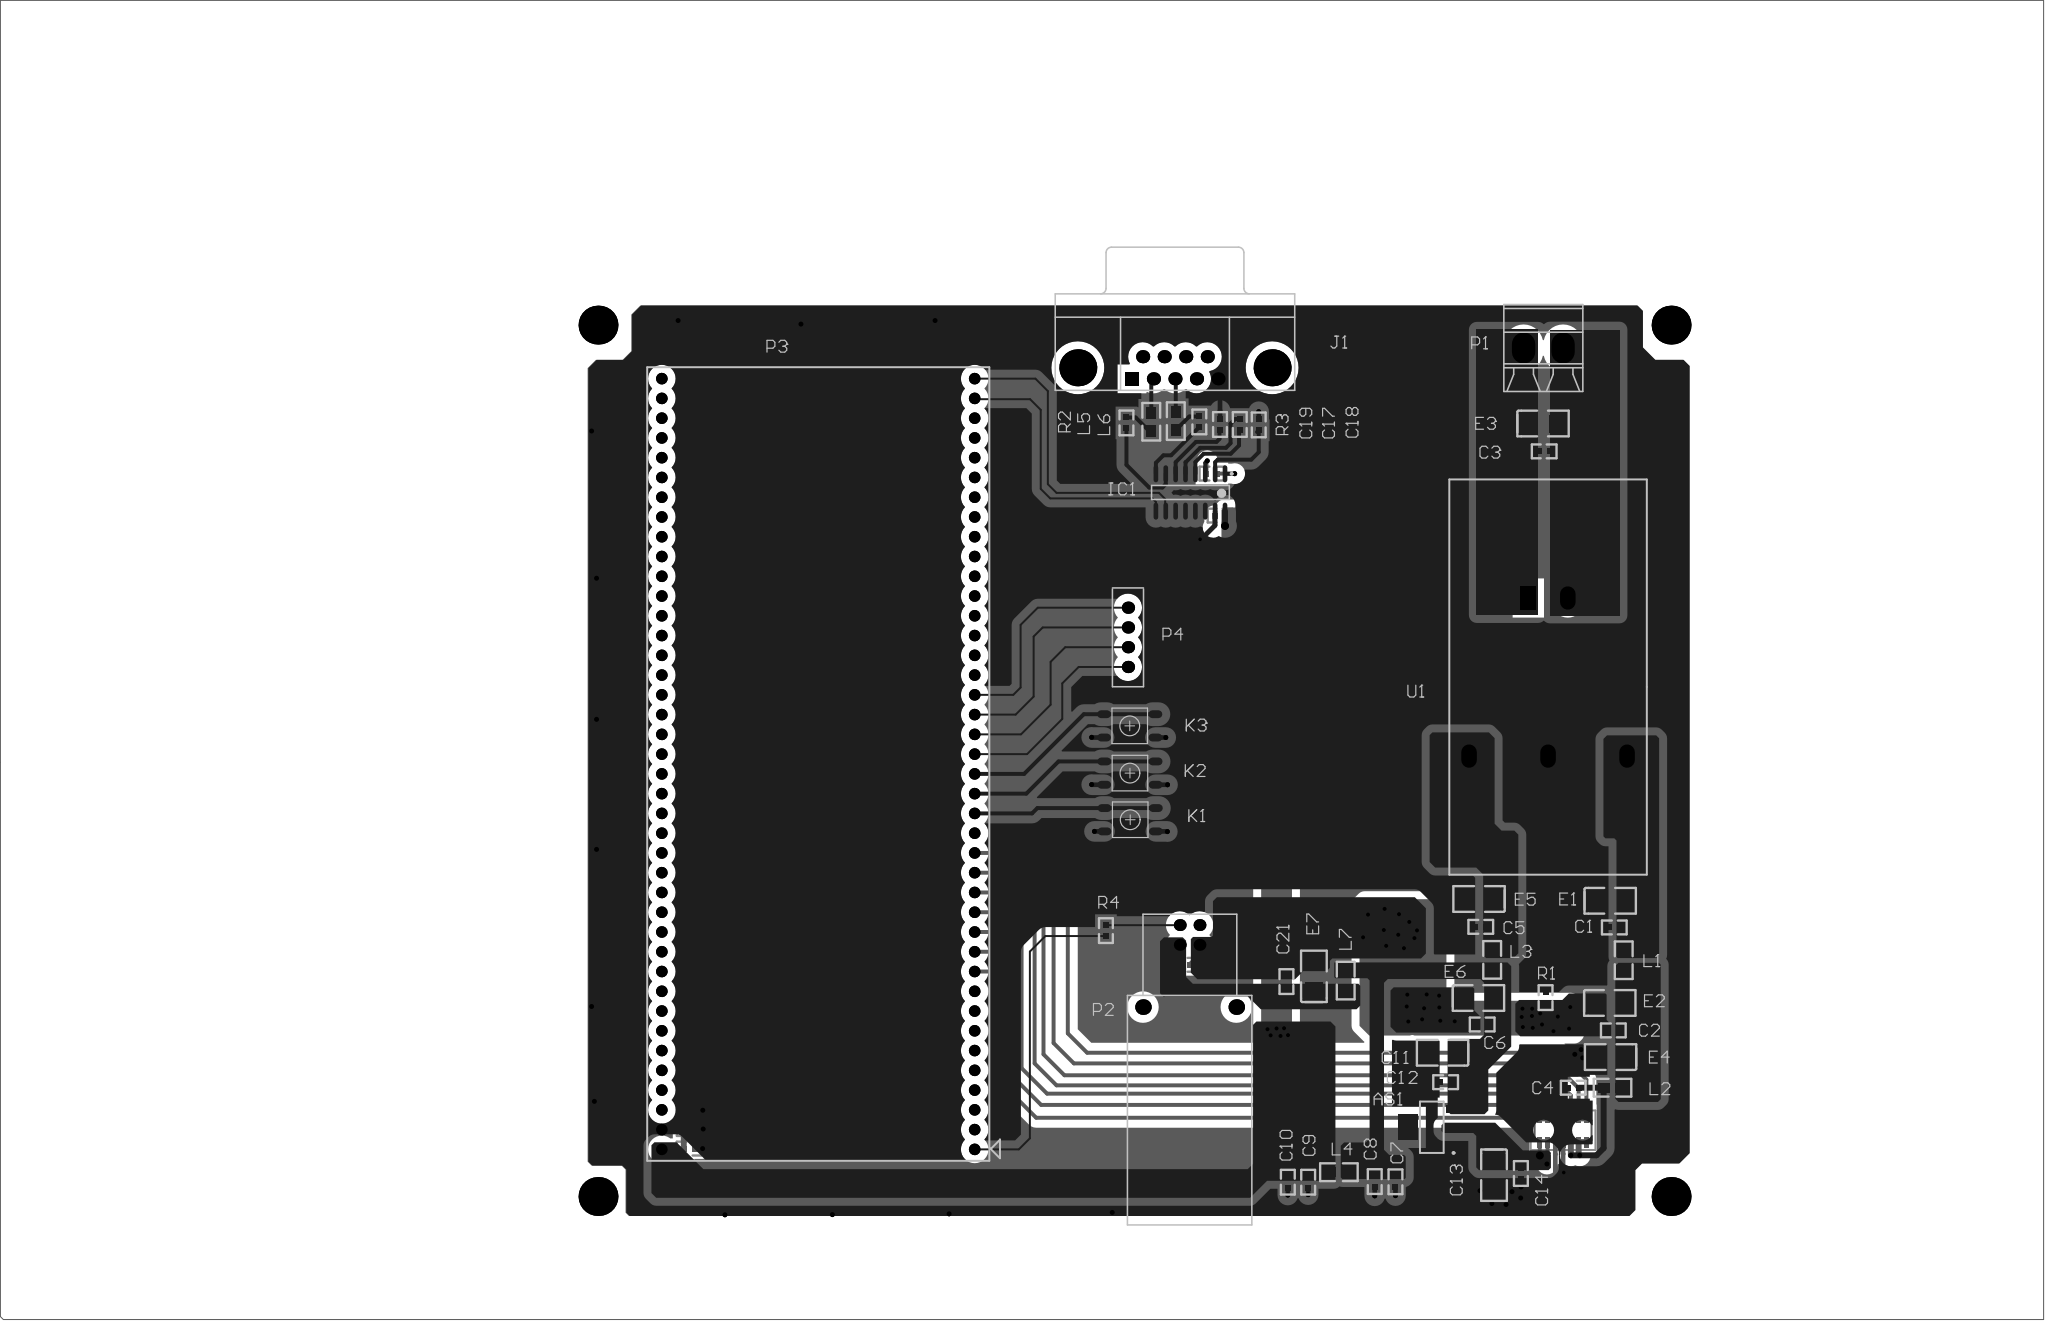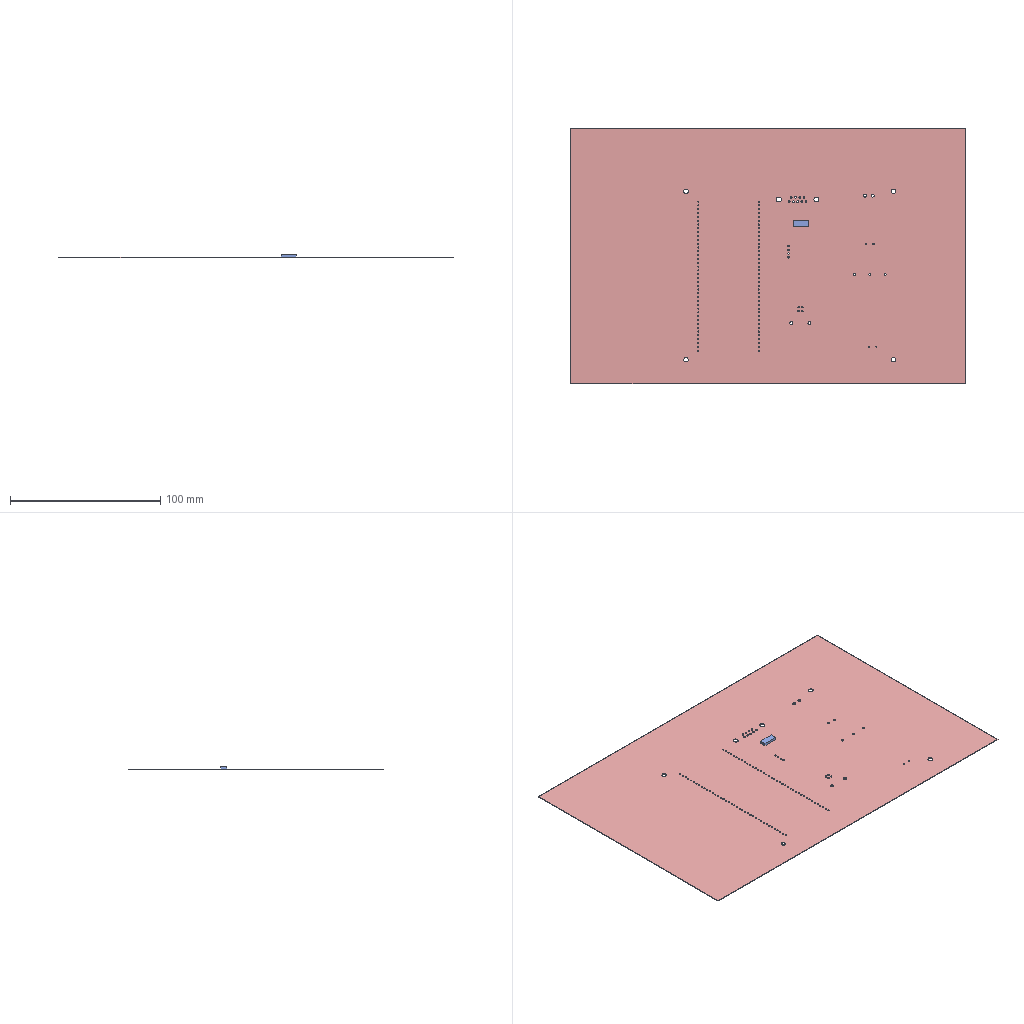Circuit board layout | Altium Designer | box 262.8 x 169.5 x 2.2 mm
Layer stack:
# Altium Designer layer stack of  (unit mm; dielectric type: 0 none, 1 core, 2 prepreg, 3 surface material)
index,name,kind,layer,copper_thickness_mm,dielectric_type,dielectric_thickness_mm,dielectric_material,dielectric_constant
0,Top Paste,other,,,,,,
1,Top Overlay,other,,,,,,
2,Top Solder,dielectric,,,3,0.0102,Solder Resist,3.5
3,Top Layer,copper,Top Layer,0.0356,,,,
4,Dielectric1,dielectric,,,1,0.32,FR-4,4.8
5,Bottom Layer,copper,Bottom Layer,0.0356,,,,
6,Bottom Solder,dielectric,,,3,0.0102,Solder Resist,3.5
7,Bottom Overlay,other,,,,,,
8,Bottom Paste,other,,,,,,
# drill layer pairs: low layer,high layer
drill_pair,Top Layer,Bottom Layer
Part placement:
Designator,Comment,Layer,Footprint,Center-X(mm),Center-Y(mm),Rotation
U1,YD10,TopLayer,YD10,126.178,70.764,270
R4,0R,TopLayer,0603,69.317,38.176,90
R3,100,TopLayer,0603,81.331,103.556,270
R2,100,TopLayer,0603,71.958,103.429,270
R1,0R,TopLayer,0603,125.857,29.566,90
P4,Header 4H,TopLayer,DIP-4,72.153,75.87,180
L7,1UH,TopLayer,0805,100.152,31.75,270
L6,600O/500mA-0805,TopLayer,0805,78.299,103.657,90
L5,600O/500mA-0805,TopLayer,0805,75.15,103.581,90
L4,1UH,TopLayer,0805,99.28,7.125,360
L3,1UH,TopLayer,0805,118.99,34.417,270
L2,1UH,TopLayer,0805,134.468,17.983,180
L1,1UH,TopLayer,0805,135.907,34.366,270
IC1,MAX3232,TopLayer,SOIC127P600-16N,80.188,94.488,270
E7,10U,TopLayer,1210,96.063,32.36,270
E6,22U,TopLayer,1210,117.288,29.515,180
E5,22U,TopLayer,1210,117.238,42.24,360
E4,22U,TopLayer,1210,134.154,21.92,360
E3,22U,TopLayer,1210,125.594,103.353,180
E2,22U,TopLayer,1210,134.179,28.88,180
E1,22U,TopLayer,1210,134.23,42.012,180
C21,0.01u,TopLayer,0603,92.532,31.623,90
C19,100n/50V,TopLayer,0603,83.989,103.226,270
C18,100n/50V,TopLayer,0603,88.967,103.175,270
C17,100n/50V,TopLayer,0603,86.529,103.226,90
C14,0.1u,TopLayer,0603,122.682,6.96,270
C13,10u,TopLayer,1210,119.228,6.68,90
C12,0.1u,TopLayer,0603,113.005,18.694,180
C11,10u,TopLayer,1210,112.547,22.479,360
C10,0.1u,TopLayer,0603,92.71,5.842,270
C9,0.1U,TopLayer,0603,95.326,5.842,90
C8,0.1U,TopLayer,0603,103.886,5.918,90
C7,0.1U,TopLayer,0603,106.553,5.893,90
C6,0.1u,TopLayer,0603,117.704,26.111,180
C5,0.1u,TopLayer,0603,117.526,38.659,180
C4,0.1u,TopLayer,0603,129.413,17.983,180
C3,0.1u,TopLayer,0603,125.679,99.771,0
C2,0.1u,TopLayer,0603,134.569,25.349,180
C1,0.1u,TopLayer,0603,134.696,38.583,180
AS1,AS117,TopLayer,SOT223-4,111.227,12.903,180
P3,Header 10X2,TopLayer,c8051,32.325,59.588,90
K3,KFC-006S-HN,TopLayer,KNOB-SMD,72.381,64.491,180
K2,KFC-006S-HN,TopLayer,KNOB-SMD,72.407,58.42,180
K1,KFC-006S-HN,TopLayer,KNOB-SMD,72.441,52.426,180
P2,PD,TopLayer,guang2,80.083,33.616,90
P1,,TopLayer,MKDS3_2RMI,125.569,113.055,90
J1,D Connector 9,TopLayer,DSUB1.385-2H9,78.198,110.515,360
LASER_1,1905LMIC,BottomLayer,CLM-107-02-H-D-K-TR,128.109,12.522,180
C24,0.1U,BottomLayer,0603,15.739,15.062,180
C23,0.1U,BottomLayer,0603,15.726,12.675,180
C22,0.1U,BottomLayer,0603,15.714,10.16,180
C20,0.1u,BottomLayer,0603,79.493,33.782,0
C16,100n/50V,BottomLayer,0603,83.998,91.516,360
C15,100n/50V,BottomLayer,0603,82.948,96.913,180
Pad and via stacks:
# Altium Designer via and pad stacks of  (unit mm). Each distinct definition once, with the count of objects using it.
# via: kind,start_layer,end_layer,hole_mm,diameter_mm,mode(0 simple;1 top-mid-bottom;2 full stack),diameter_per_layer,count,example_net
# pad: kind,layer,hole_mm,hole_type(0 round;1 square;2 slot),plating,top_size,top_shape(1 round;2 rect;3 octagon;9 rounded rect),mid_size,bottom_size,mode,footprint,size_per_layer,count,example
pad,Top Layer,0,0,plated,0.762x0.762,2,0.762x0.762,0.762x0.762,0,0603,,40,C4.1
pad,Top Layer,0,0,plated,1.524x1.27,2,1.524x1.27,1.524x1.27,0,0805,,14,L2.1
pad,Top Layer,0,0,plated,1.905x2.286,2,1.905x2.286,1.905x2.286,0,1210,,18,E4.1
pad,Top Layer,0,0,plated,2.54x1.016,2,2.54x1.016,2.54x1.016,0,SOT223-4,,3,AS1.1
pad,Top Layer,0,0,plated,2.54x3.302,2,2.54x3.302,2.54x3.302,0,SOT223-4,,1,AS1.4
pad,Top Layer,0,0,plated,1.778x1.016,1,1.778x1.016,1.778x1.016,0,KNOB-SMD,,12,K1.1
pad,Top Layer,0,0,plated,0.6x2.2,1,0.6x2.2,0.6x2.2,0,SOIC127P600-16N,,16,IC1.1
pad,Bottom Layer,0,0,unplated,1.37x0.61,2,1.37x0.61,1.37x0.61,0,CLM-107-02-H-D-K-TR,,14,LASER_1.1
pad,Bottom Layer,0,0,plated,0.762x0.762,2,0.762x0.762,0.762x0.762,0,0603,,12,C22.1
pad,Multi-Layer,3.26,0,plated,4.76x4.76,1,4.76x4.76,4.76x4.76,0,DSUB1.385-2H9,,2,J1.11
pad,Multi-Layer,1.09,0,plated,1.69x1.69,2,1.69x1.69,1.69x1.69,0,DSUB1.385-2H9,,1,J1.1
pad,Multi-Layer,1.09,0,plated,1.69x1.69,1,1.69x1.69,1.69x1.69,0,DSUB1.385-2H9,,8,J1.6
pad,Multi-Layer,0.635,0,unplated,0x0,1,0x0,0x0,1,CLM-107-02-H-D-K-TR,,2,LASER_1.15
pad,Multi-Layer,0.889,0,plated,1.575x1.575,1,1.575x1.575,1.575x1.575,0,DIP-4,,4,P4.1
pad,Multi-Layer,1.3,0,plated,3x2,1,3x2,3x2,0,YD10,,4,U1.5
pad,Multi-Layer,1.3,0,plated,3x2,2,3x2,3x2,0,YD10,,1,U1.1
pad,Multi-Layer,0.762,0,plated,1.504x1.5,1,1.504x1.5,1.504x1.5,0,c8051,,80,P3.80
pad,Multi-Layer,3,0,plated,5x5,1,5x5,5x5,0,,,4,0
pad,Multi-Layer,2,0,plated,3x4,1,3x4,3x4,0,MKDS3_2RMI,,2,P1.2
pad,Multi-Layer,0.9,0,plated,1.524x1.524,1,1.524x1.524,1.524x1.524,0,guang2,,4,P2.4
pad,Multi-Layer,2,0,plated,2x2,1,2x2,2x2,0,guang2,,2,P2.
via,Top Layer,Bottom Layer,0.254,0.4572,0,,2,GND
via,Top Layer,Bottom Layer,0.381,0.635,0,,41,VCC-5V
via,Top Layer,Bottom Layer,0.254,0.508,0,,39,AGND
via,Top Layer,Bottom Layer,0.508,1.016,0,,2,5VD_MCU
Copper pours:
name,layer,net,type(0 solid;1 hatched;2 none)
Top Layer-No Net,Top Layer,GND,0
Top Layer-No Net,Top Layer,AGND,0
Top Layer-No Net,Top Layer,AGND,0
Top Layer-No Net,Top Layer,AGND,0
Top Layer-No Net,Top Layer,5VD_MCU,0
Top Layer-No Net,Top Layer,+5V,0
Top Layer-No Net,Top Layer,3.3V,0
TopLayer-No Net,Top Layer,+5V1,0
TopLayer-No Net,Top Layer,-5V1,0
TopLayer-No Net,Top Layer,NetC20_1,0
TopLayer-No Net,Top Layer,-5V,0
Top Layer-No Net,Bottom Layer,GND,0
Top Layer-No Net,Bottom Layer,AGND,0
Top Layer-No Net,Bottom Layer,5VD_MCU,0
Design rules, without the lines most boards share:
# Altium Designer design rules of  (exported by Altium Designer, unit mm)
# columns: name | kind | enabled | priority | scope1 | scope2 | descriptor | typed fields (field=value)
SolderMaskExpansion_1 | 13 | enabled | 1 | IsVia | All | Solder Mask Expansion (Expansion =-40mil) (IsVia) | expansion=-1.016
PlaneConnect_1 | 6 | enabled | 1 | (InPadClass('All Pads')) | All | Power Plane Connect Rule(Relief Connect )(Expansion=20mil) (Conductor Width=10mil) (Air Gap=10mil) (Entries=4) ((InPadClass('All Pads'))) | relief_conductor_width=0.254 relief_entries=4 relief_expansion=0.508
DiffPairsRouting | 51 | enabled | 1 | All | All | Differential Pairs Uncoupled Length using the Gap Constraints (Min=10mil) (Max=10mil) (Prefered=10mil)  and Width Constraints (Min=15mil) (Max=15mil) (Prefered=15mil) (All) |
HoleSize | 42 | disabled | 1 | All | All | Hole Size Constraint (Min=1mil) (Max=100mil) (Disabled)(All) |
ComponentClearance | 24 | disabled | 1 | All | All | Component Clearance Constraint ( Horizontal Gap = 10mil, Vertical Gap = 10mil ) (Disabled)(All),(All)  | gap=0.254
Testpoint | 43 | enabled | 1 | (IsPad And (OnTopLayer Or OnBottomLayer)) | All | Fabrication Testpoint Style (Under Component=Yes) ((IsPad And (OnTopLayer Or OnBottomLayer))) |
TestPointUsage | 44 | enabled | 1 | All | All | Fabrication Testpoint Usage (Valid =One Required, Allow multiple per net=No) (All) |
SolderMaskExpansion | 13 | enabled | 2 | All | All | Solder Mask Expansion (Expansion =2mil) (All) | expansion=0.0508
PasteMaskExpansion | 14 | enabled | 1 | All | All | Paste Mask Expansion (Expansion =0mil) (All) | expansion=0
RoutingVias | 11 | enabled | 1 | All | All | Routing Via (MinHoleWidth=10mil) (MaxHoleWidth=15mil) (PreferredHoleWidth=10mil) (MinWidth=18mil) (MaxWidth=25mil) (PreferedWidth=18mil) (All) | via_min_hole=0.254 via_max_hole=0.381 via_preferred_diameter=0.4572 via_preferred_hole=0.254
Width | 2 | enabled | 1 | All | All | Width Constraint (Min=8mil) (Max=200mil) (Preferred=10mil) (All) |
PolygonConnect | 20 | enabled | 2 | All | All | Polygon Connect Rule(Direct Connect )(Conductor Width=10mil) (Relief Angle=90 Angle) (Entries=4) (Air Gap Width=10mil) (All),(All) | connect_style(0=relief,1=direct,2=none)=1 relief_conductor_width=0.254 relief_entries=4
PlaneConnect | 6 | enabled | 2 | All | All | Power Plane Connect Rule(Direct Connect )(Expansion=20mil) (Conductor Width=20mil) (Air Gap=20mil) (Entries=4) (All) | relief_conductor_width=0.508 relief_entries=4 relief_expansion=0.508
Clearance | 0 | enabled | 1 | All | All | Clearance Constraint (Gap=10mil) (All),(All) | gap=0.254
PolygonConnect_1 | 20 | enabled | 1 | (InPadClass('All Pads')) | All | Polygon Connect Rule(Direct Connect )(Conductor Width=20mil) (Relief Angle=90 Angle) (Entries=4) (Air Gap Width=10mil) ((InPadClass('All Pads'))),(All) | connect_style(0=relief,1=direct,2=none)=1 relief_conductor_width=0.508 relief_entries=4
HoleToHoleClearance | 52 | enabled | 1 | All | All | Hole To Hole Clearance (Gap=10mil) (All),(All) | gap=0.254
SilkscreenOverComponentPads | 54 | enabled | 1 | IsPad | All | Silk To Solder Mask (Clearance=10mil) (IsPad),(All) |
Classes set for this board:
# Altium Designer classes of  (member kind: 0 net, 1 component, 2 from-to, 3 pad, 4 layer, 5 differential pair, 6 design channel, 7 polygon, 8 structure, 9 xSignal)
# columns: class name | member kind | superclass | members
MCU-1 | 1 | no | IC1; C33; C16; C17; C18; C19; C20; C22; C23; C31; C32; E7; J1; K1; K2; K3; L6; L7; L8; LASER_1; P2; P3; P3; R2; R3; R4; C15; C16; C17; C18; C19; C20; C21; C22; C23; C24; E7; IC1; L5; L6; L7; P4; R2; R3; R4;
LD-1 | 1 | no | C1; C2; C3; C4; C5; C6; C7; C8; C9; C10; C11; C12; C13; C14; E1; E2; E3; E4; E5; E6; L1; L2; L3; L4; P1; R1; U1; AS1; C1; C2; C3; C4; C5; C6; C7; C8; C9; C10; C11; C12; C13; C14; E1; E2; E3; E4; E5; E6; L1; L2; L3; L4; R1; U1;